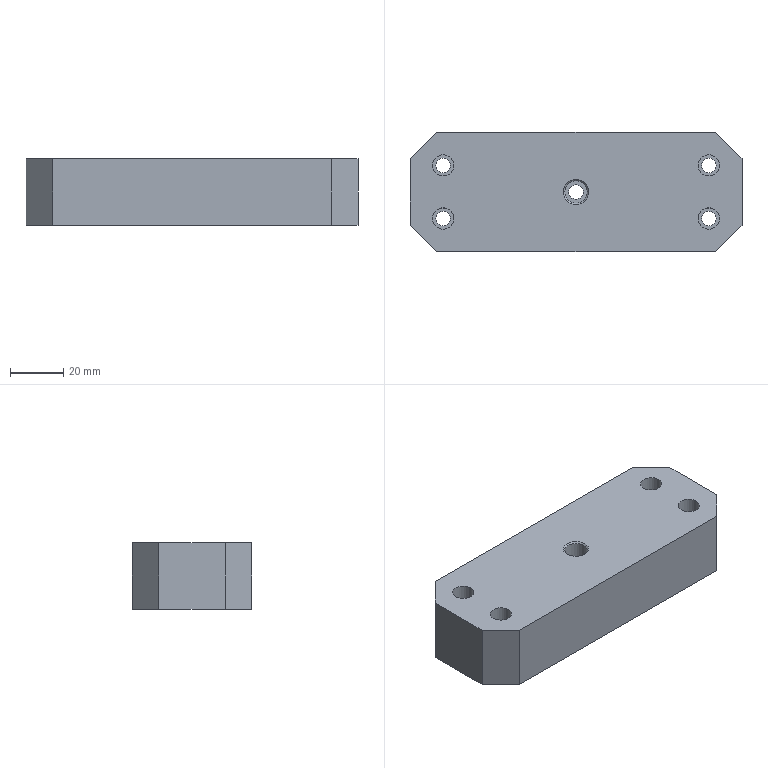Part | STEP file | Tube feed_id922_x_t | 1 solid | 34 faces | box 125 x 45 x 25 mm | volume 129874 mm3 | plane 19 | cylinder 14 | cone 1 | commonest cylinder face diameters 5.5 x5 8.5 x5 8 x4